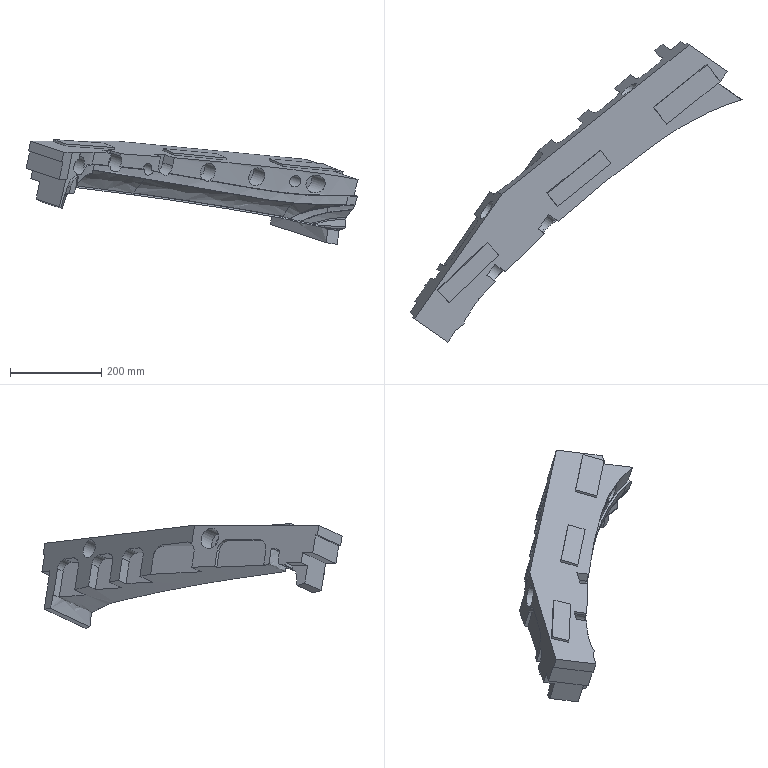Part | NX | features solid 2 | 1 solid | 194 faces | box 726.125 x 656.312 x 229.463 mm | volume 8602757 mm3 | spline 106 | plane 68 | cylinder 20 | commonest cylinder face diameters 40 x13 50 x4 25.4 x2 46 x1